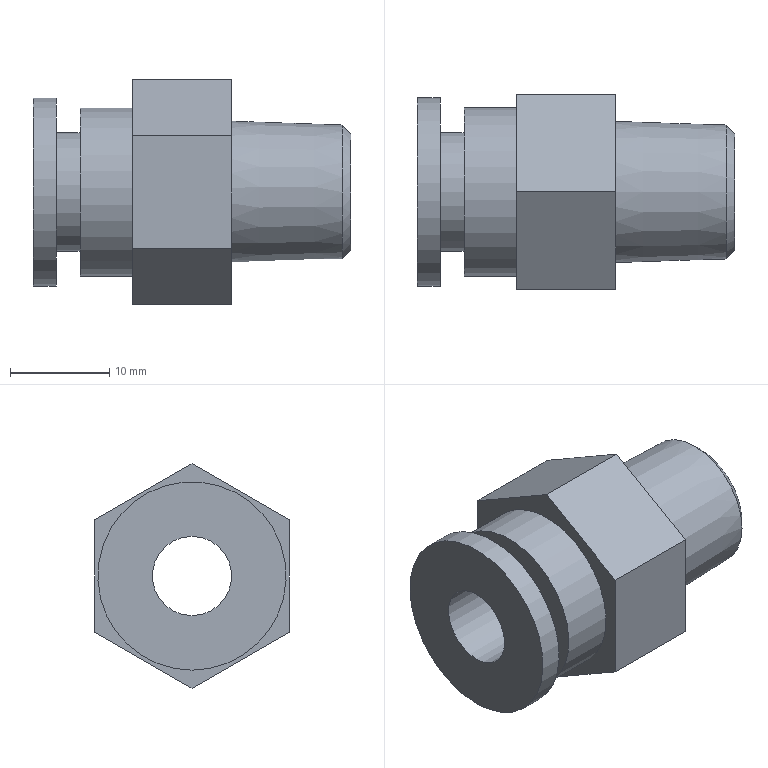Part | NX | features solid 2 | 1 solid | 18 faces | box 32 x 19.63 x 22.667 mm | volume 5655 mm3 | plane 12 | cylinder 4 | cone 2 | commonest cylinder face diameters 8 x1 12 x1 17 x1 19 x1
STEP:
#1=CARTESIAN_POINT('',(-113.,-72.,-29.095));
#2=VERTEX_POINT('',#1);
#3=CARTESIAN_POINT('',(-113.,-72.,-35.));
#4=DIRECTION('',(1.,0.,0.));
#5=DIRECTION('',(0.,0.,1.));
#6=AXIS2_PLACEMENT_3D('',#3,#4,#5);
#7=CIRCLE('',#6,5.905);
#8=EDGE_CURVE('',#2,#2,#7,.T.);
#9=ORIENTED_EDGE('',*,*,#8,.T.);
#10=EDGE_LOOP('',(#9));
#11=FACE_BOUND('',#10,.T.);
#12=CARTESIAN_POINT('',(-113.,-72.,-39.));
#13=VERTEX_POINT('',#12);
#14=CARTESIAN_POINT('',(-113.,-72.,-35.));
#15=DIRECTION('',(1.,0.,0.));
#16=DIRECTION('',(0.,0.,-1.));
#17=AXIS2_PLACEMENT_3D('',#14,#15,#16);
#18=CIRCLE('',#17,4.);
#19=EDGE_CURVE('',#13,#13,#18,.T.);
#20=ORIENTED_EDGE('',*,*,#19,.F.);
#21=EDGE_LOOP('',(#20));
#22=FACE_BOUND('',#21,.T.);
#23=CARTESIAN_POINT('',(-113.,-72.,-35.));
#24=DIRECTION('',(1.,0.,0.));
#25=DIRECTION('',(0.,0.,1.));
#26=AXIS2_PLACEMENT_3D('',#23,#24,#25);
#27=PLANE('',#26);
#28=ADVANCED_FACE('',(#11,#22),#27,.T.);
#29=CARTESIAN_POINT('',(-145.,-72.,-44.5));
#30=VERTEX_POINT('',#29);
#31=CARTESIAN_POINT('',(-145.,-72.,-35.));
#32=DIRECTION('',(-1.,0.,0.));
#33=DIRECTION('',(0.,0.,-1.));
#34=AXIS2_PLACEMENT_3D('',#31,#32,#33);
#35=CIRCLE('',#34,9.5);
#36=EDGE_CURVE('',#30,#30,#35,.T.);
#37=ORIENTED_EDGE('',*,*,#36,.T.);
#38=EDGE_LOOP('',(#37));
#39=FACE_BOUND('',#38,.T.);
#40=CARTESIAN_POINT('',(-145.,-72.,-39.));
#41=VERTEX_POINT('',#40);
#42=CARTESIAN_POINT('',(-145.,-72.,-35.));
#43=DIRECTION('',(-1.,0.,0.));
#44=DIRECTION('',(0.,0.,-1.));
#45=AXIS2_PLACEMENT_3D('',#42,#43,#44);
#46=CIRCLE('',#45,4.);
#47=EDGE_CURVE('',#41,#41,#46,.T.);
#48=ORIENTED_EDGE('',*,*,#47,.F.);
#49=EDGE_LOOP('',(#48));
#50=FACE_BOUND('',#49,.T.);
#51=CARTESIAN_POINT('',(-145.,-72.,-35.));
#52=DIRECTION('',(-1.,0.,0.));
#53=DIRECTION('',(0.,0.,-1.));
#54=AXIS2_PLACEMENT_3D('',#51,#52,#53);
#55=PLANE('',#54);
#56=ADVANCED_FACE('',(#39,#50),#55,.T.);
#57=ORIENTED_EDGE('',*,*,#8,.F.);
#58=EDGE_LOOP('',(#57));
#59=FACE_BOUND('',#58,.T.);
#60=CARTESIAN_POINT('',(-113.86,-72.,-28.24));
#61=VERTEX_POINT('',#60);
#62=CARTESIAN_POINT('',(-113.86,-72.,-35.));
#63=DIRECTION('',(1.,0.,0.));
#64=DIRECTION('',(0.,0.,1.));
#65=AXIS2_PLACEMENT_3D('',#62,#63,#64);
#66=CIRCLE('',#65,6.76);
#67=EDGE_CURVE('',#61,#61,#66,.T.);
#68=ORIENTED_EDGE('',*,*,#67,.T.);
#69=EDGE_LOOP('',(#68));
#70=FACE_BOUND('',#69,.T.);
#71=CARTESIAN_POINT('',(-113.,-72.,-35.));
#72=DIRECTION('',(-1.,0.,0.));
#73=DIRECTION('',(0.,0.,1.));
#74=AXIS2_PLACEMENT_3D('',#71,#72,#73);
#75=CONICAL_SURFACE('',#74,5.905,0.7825);
#76=ADVANCED_FACE('',(#59,#70),#75,.T.);
#77=ORIENTED_EDGE('',*,*,#67,.F.);
#78=EDGE_LOOP('',(#77));
#79=FACE_BOUND('',#78,.T.);
#80=CARTESIAN_POINT('',(-125.,-72.,-27.86));
#81=VERTEX_POINT('',#80);
#82=CARTESIAN_POINT('',(-125.,-72.,-35.));
#83=DIRECTION('',(-1.,0.,0.));
#84=DIRECTION('',(0.,0.,1.));
#85=AXIS2_PLACEMENT_3D('',#82,#83,#84);
#86=CIRCLE('',#85,7.14);
#87=EDGE_CURVE('',#81,#81,#86,.T.);
#88=ORIENTED_EDGE('',*,*,#87,.F.);
#89=EDGE_LOOP('',(#88));
#90=FACE_BOUND('',#89,.T.);
#91=CARTESIAN_POINT('',(-113.86,-72.,-35.));
#92=DIRECTION('',(-1.,0.,0.));
#93=DIRECTION('',(0.,0.,1.));
#94=AXIS2_PLACEMENT_3D('',#91,#92,#93);
#95=CONICAL_SURFACE('',#94,6.76,0.0341);
#96=ADVANCED_FACE('',(#79,#90),#95,.T.);
#97=CARTESIAN_POINT('',(-125.,-72.,-46.333));
#98=VERTEX_POINT('',#97);
#99=CARTESIAN_POINT('',(-125.,-62.185,-40.667));
#100=VERTEX_POINT('',#99);
#101=CARTESIAN_POINT('',(-125.,-72.,-46.333));
#102=DIRECTION('',(0.,0.866,0.5));
#103=VECTOR('',#102,1000.);
#104=LINE('',#101,#103);
#105=EDGE_CURVE('',#98,#100,#104,.T.);
#106=ORIENTED_EDGE('',*,*,#105,.T.);
#107=CARTESIAN_POINT('',(-125.,-62.185,-29.333));
#108=VERTEX_POINT('',#107);
#109=CARTESIAN_POINT('',(-125.,-62.185,-40.667));
#110=DIRECTION('',(0.,0.,1.));
#111=VECTOR('',#110,1000.);
#112=LINE('',#109,#111);
#113=EDGE_CURVE('',#100,#108,#112,.T.);
#114=ORIENTED_EDGE('',*,*,#113,.T.);
#115=CARTESIAN_POINT('',(-125.,-72.,-23.667));
#116=VERTEX_POINT('',#115);
#117=CARTESIAN_POINT('',(-125.,-62.185,-29.333));
#118=DIRECTION('',(0.,-0.866,0.5));
#119=VECTOR('',#118,1000.);
#120=LINE('',#117,#119);
#121=EDGE_CURVE('',#108,#116,#120,.T.);
#122=ORIENTED_EDGE('',*,*,#121,.T.);
#123=CARTESIAN_POINT('',(-125.,-81.815,-29.333));
#124=VERTEX_POINT('',#123);
#125=CARTESIAN_POINT('',(-125.,-72.,-23.667));
#126=DIRECTION('',(0.,-0.866,-0.5));
#127=VECTOR('',#126,1000.);
#128=LINE('',#125,#127);
#129=EDGE_CURVE('',#116,#124,#128,.T.);
#130=ORIENTED_EDGE('',*,*,#129,.T.);
#131=CARTESIAN_POINT('',(-125.,-81.815,-40.667));
#132=VERTEX_POINT('',#131);
#133=CARTESIAN_POINT('',(-125.,-81.815,-29.333));
#134=DIRECTION('',(0.,0.,-1.));
#135=VECTOR('',#134,1000.);
#136=LINE('',#133,#135);
#137=EDGE_CURVE('',#124,#132,#136,.T.);
#138=ORIENTED_EDGE('',*,*,#137,.T.);
#139=CARTESIAN_POINT('',(-125.,-81.815,-40.667));
#140=DIRECTION('',(0.,0.866,-0.5));
#141=VECTOR('',#140,1000.);
#142=LINE('',#139,#141);
#143=EDGE_CURVE('',#132,#98,#142,.T.);
#144=ORIENTED_EDGE('',*,*,#143,.T.);
#145=EDGE_LOOP('',(#106,#114,#122,#130,#138,#144));
#146=FACE_BOUND('',#145,.T.);
#147=ORIENTED_EDGE('',*,*,#87,.T.);
#148=EDGE_LOOP('',(#147));
#149=FACE_BOUND('',#148,.T.);
#150=CARTESIAN_POINT('',(-125.,-72.,-35.));
#151=DIRECTION('',(1.,0.,0.));
#152=DIRECTION('',(0.,0.,1.));
#153=AXIS2_PLACEMENT_3D('',#150,#151,#152);
#154=PLANE('',#153);
#155=ADVANCED_FACE('',(#146,#149),#154,.T.);
#156=CARTESIAN_POINT('',(-135.,-81.815,-40.667));
#157=VERTEX_POINT('',#156);
#158=CARTESIAN_POINT('',(-135.,-72.,-46.333));
#159=VERTEX_POINT('',#158);
#160=CARTESIAN_POINT('',(-135.,-81.815,-40.667));
#161=DIRECTION('',(0.,0.866,-0.5));
#162=VECTOR('',#161,1000.);
#163=LINE('',#160,#162);
#164=EDGE_CURVE('',#157,#159,#163,.T.);
#165=ORIENTED_EDGE('',*,*,#164,.T.);
#166=CARTESIAN_POINT('',(-125.,-72.,-46.333));
#167=DIRECTION('',(-1.,0.,0.));
#168=VECTOR('',#167,1000.);
#169=LINE('',#166,#168);
#170=EDGE_CURVE('',#98,#159,#169,.T.);
#171=ORIENTED_EDGE('',*,*,#170,.F.);
#172=ORIENTED_EDGE('',*,*,#143,.F.);
#173=CARTESIAN_POINT('',(-125.,-81.815,-40.667));
#174=DIRECTION('',(-1.,0.,0.));
#175=VECTOR('',#174,1000.);
#176=LINE('',#173,#175);
#177=EDGE_CURVE('',#132,#157,#176,.T.);
#178=ORIENTED_EDGE('',*,*,#177,.T.);
#179=EDGE_LOOP('',(#165,#171,#172,#178));
#180=FACE_BOUND('',#179,.T.);
#181=CARTESIAN_POINT('',(-130.,-76.907,-43.5));
#182=DIRECTION('',(0.,-0.5,-0.866));
#183=DIRECTION('',(0.,0.866,-0.5));
#184=AXIS2_PLACEMENT_3D('',#181,#182,#183);
#185=PLANE('',#184);
#186=ADVANCED_FACE('',(#180),#185,.T.);
#187=CARTESIAN_POINT('',(-135.,-81.815,-29.333));
#188=VERTEX_POINT('',#187);
#189=CARTESIAN_POINT('',(-135.,-81.815,-29.333));
#190=DIRECTION('',(0.,0.,-1.));
#191=VECTOR('',#190,1000.);
#192=LINE('',#189,#191);
#193=EDGE_CURVE('',#188,#157,#192,.T.);
#194=ORIENTED_EDGE('',*,*,#193,.T.);
#195=ORIENTED_EDGE('',*,*,#177,.F.);
#196=ORIENTED_EDGE('',*,*,#137,.F.);
#197=CARTESIAN_POINT('',(-125.,-81.815,-29.333));
#198=DIRECTION('',(-1.,0.,0.));
#199=VECTOR('',#198,1000.);
#200=LINE('',#197,#199);
#201=EDGE_CURVE('',#124,#188,#200,.T.);
#202=ORIENTED_EDGE('',*,*,#201,.T.);
#203=EDGE_LOOP('',(#194,#195,#196,#202));
#204=FACE_BOUND('',#203,.T.);
#205=CARTESIAN_POINT('',(-130.,-81.815,-35.));
#206=DIRECTION('',(0.,-1.,0.));
#207=DIRECTION('',(0.,0.,-1.));
#208=AXIS2_PLACEMENT_3D('',#205,#206,#207);
#209=PLANE('',#208);
#210=ADVANCED_FACE('',(#204),#209,.T.);
#211=CARTESIAN_POINT('',(-135.,-72.,-23.667));
#212=VERTEX_POINT('',#211);
#213=CARTESIAN_POINT('',(-135.,-72.,-23.667));
#214=DIRECTION('',(0.,-0.866,-0.5));
#215=VECTOR('',#214,1000.);
#216=LINE('',#213,#215);
#217=EDGE_CURVE('',#212,#188,#216,.T.);
#218=ORIENTED_EDGE('',*,*,#217,.T.);
#219=ORIENTED_EDGE('',*,*,#201,.F.);
#220=ORIENTED_EDGE('',*,*,#129,.F.);
#221=CARTESIAN_POINT('',(-125.,-72.,-23.667));
#222=DIRECTION('',(-1.,0.,0.));
#223=VECTOR('',#222,1000.);
#224=LINE('',#221,#223);
#225=EDGE_CURVE('',#116,#212,#224,.T.);
#226=ORIENTED_EDGE('',*,*,#225,.T.);
#227=EDGE_LOOP('',(#218,#219,#220,#226));
#228=FACE_BOUND('',#227,.T.);
#229=CARTESIAN_POINT('',(-130.,-76.907,-26.5));
#230=DIRECTION('',(0.,-0.5,0.866));
#231=DIRECTION('',(0.,-0.866,-0.5));
#232=AXIS2_PLACEMENT_3D('',#229,#230,#231);
#233=PLANE('',#232);
#234=ADVANCED_FACE('',(#228),#233,.T.);
#235=CARTESIAN_POINT('',(-135.,-62.185,-29.333));
#236=VERTEX_POINT('',#235);
#237=CARTESIAN_POINT('',(-135.,-62.185,-29.333));
#238=DIRECTION('',(0.,-0.866,0.5));
#239=VECTOR('',#238,1000.);
#240=LINE('',#237,#239);
#241=EDGE_CURVE('',#236,#212,#240,.T.);
#242=ORIENTED_EDGE('',*,*,#241,.T.);
#243=ORIENTED_EDGE('',*,*,#225,.F.);
#244=ORIENTED_EDGE('',*,*,#121,.F.);
#245=CARTESIAN_POINT('',(-125.,-62.185,-29.333));
#246=DIRECTION('',(-1.,0.,0.));
#247=VECTOR('',#246,1000.);
#248=LINE('',#245,#247);
#249=EDGE_CURVE('',#108,#236,#248,.T.);
#250=ORIENTED_EDGE('',*,*,#249,.T.);
#251=EDGE_LOOP('',(#242,#243,#244,#250));
#252=FACE_BOUND('',#251,.T.);
#253=CARTESIAN_POINT('',(-130.,-67.093,-26.5));
#254=DIRECTION('',(0.,0.5,0.866));
#255=DIRECTION('',(0.,-0.866,0.5));
#256=AXIS2_PLACEMENT_3D('',#253,#254,#255);
#257=PLANE('',#256);
#258=ADVANCED_FACE('',(#252),#257,.T.);
#259=CARTESIAN_POINT('',(-135.,-62.185,-40.667));
#260=VERTEX_POINT('',#259);
#261=CARTESIAN_POINT('',(-135.,-62.185,-40.667));
#262=DIRECTION('',(0.,0.,1.));
#263=VECTOR('',#262,1000.);
#264=LINE('',#261,#263);
#265=EDGE_CURVE('',#260,#236,#264,.T.);
#266=ORIENTED_EDGE('',*,*,#265,.T.);
#267=ORIENTED_EDGE('',*,*,#249,.F.);
#268=ORIENTED_EDGE('',*,*,#113,.F.);
#269=CARTESIAN_POINT('',(-125.,-62.185,-40.667));
#270=DIRECTION('',(-1.,0.,0.));
#271=VECTOR('',#270,1000.);
#272=LINE('',#269,#271);
#273=EDGE_CURVE('',#100,#260,#272,.T.);
#274=ORIENTED_EDGE('',*,*,#273,.T.);
#275=EDGE_LOOP('',(#266,#267,#268,#274));
#276=FACE_BOUND('',#275,.T.);
#277=CARTESIAN_POINT('',(-130.,-62.185,-35.));
#278=DIRECTION('',(0.,1.,0.));
#279=DIRECTION('',(1.,0.,0.));
#280=AXIS2_PLACEMENT_3D('',#277,#278,#279);
#281=PLANE('',#280);
#282=ADVANCED_FACE('',(#276),#281,.T.);
#283=CARTESIAN_POINT('',(-135.,-72.,-46.333));
#284=DIRECTION('',(0.,0.866,0.5));
#285=VECTOR('',#284,1000.);
#286=LINE('',#283,#285);
#287=EDGE_CURVE('',#159,#260,#286,.T.);
#288=ORIENTED_EDGE('',*,*,#287,.T.);
#289=ORIENTED_EDGE('',*,*,#273,.F.);
#290=ORIENTED_EDGE('',*,*,#105,.F.);
#291=ORIENTED_EDGE('',*,*,#170,.T.);
#292=EDGE_LOOP('',(#288,#289,#290,#291));
#293=FACE_BOUND('',#292,.T.);
#294=CARTESIAN_POINT('',(-130.,-67.093,-43.5));
#295=DIRECTION('',(0.,0.5,-0.866));
#296=DIRECTION('',(0.,0.866,0.5));
#297=AXIS2_PLACEMENT_3D('',#294,#295,#296);
#298=PLANE('',#297);
#299=ADVANCED_FACE('',(#293),#298,.T.);
#300=CARTESIAN_POINT('',(-135.,-72.,-43.5));
#301=VERTEX_POINT('',#300);
#302=CARTESIAN_POINT('',(-135.,-72.,-35.));
#303=DIRECTION('',(1.,0.,0.));
#304=DIRECTION('',(0.,0.,-1.));
#305=AXIS2_PLACEMENT_3D('',#302,#303,#304);
#306=CIRCLE('',#305,8.5);
#307=EDGE_CURVE('',#301,#301,#306,.T.);
#308=ORIENTED_EDGE('',*,*,#307,.T.);
#309=EDGE_LOOP('',(#308));
#310=FACE_BOUND('',#309,.T.);
#311=ORIENTED_EDGE('',*,*,#193,.F.);
#312=ORIENTED_EDGE('',*,*,#217,.F.);
#313=ORIENTED_EDGE('',*,*,#241,.F.);
#314=ORIENTED_EDGE('',*,*,#265,.F.);
#315=ORIENTED_EDGE('',*,*,#287,.F.);
#316=ORIENTED_EDGE('',*,*,#164,.F.);
#317=EDGE_LOOP('',(#311,#312,#313,#314,#315,#316));
#318=FACE_BOUND('',#317,.T.);
#319=CARTESIAN_POINT('',(-135.,-72.,-35.));
#320=DIRECTION('',(-1.,0.,0.));
#321=DIRECTION('',(0.,0.,-1.));
#322=AXIS2_PLACEMENT_3D('',#319,#320,#321);
#323=PLANE('',#322);
#324=ADVANCED_FACE('',(#310,#318),#323,.T.);
#325=CARTESIAN_POINT('',(-140.3,-72.,-41.));
#326=VERTEX_POINT('',#325);
#327=CARTESIAN_POINT('',(-140.3,-72.,-35.));
#328=DIRECTION('',(1.,0.,0.));
#329=DIRECTION('',(0.,0.,-1.));
#330=AXIS2_PLACEMENT_3D('',#327,#328,#329);
#331=CIRCLE('',#330,6.);
#332=EDGE_CURVE('',#326,#326,#331,.T.);
#333=ORIENTED_EDGE('',*,*,#332,.T.);
#334=EDGE_LOOP('',(#333));
#335=FACE_BOUND('',#334,.T.);
#336=CARTESIAN_POINT('',(-140.3,-72.,-43.5));
#337=VERTEX_POINT('',#336);
#338=CARTESIAN_POINT('',(-140.3,-72.,-35.));
#339=DIRECTION('',(-1.,0.,0.));
#340=DIRECTION('',(0.,0.,-1.));
#341=AXIS2_PLACEMENT_3D('',#338,#339,#340);
#342=CIRCLE('',#341,8.5);
#343=EDGE_CURVE('',#337,#337,#342,.T.);
#344=ORIENTED_EDGE('',*,*,#343,.T.);
#345=EDGE_LOOP('',(#344));
#346=FACE_BOUND('',#345,.T.);
#347=CARTESIAN_POINT('',(-140.3,-72.,-35.));
#348=DIRECTION('',(-1.,0.,0.));
#349=DIRECTION('',(0.,0.,-1.));
#350=AXIS2_PLACEMENT_3D('',#347,#348,#349);
#351=PLANE('',#350);
#352=ADVANCED_FACE('',(#335,#346),#351,.T.);
#353=ORIENTED_EDGE('',*,*,#343,.F.);
#354=EDGE_LOOP('',(#353));
#355=FACE_BOUND('',#354,.T.);
#356=ORIENTED_EDGE('',*,*,#307,.F.);
#357=EDGE_LOOP('',(#356));
#358=FACE_BOUND('',#357,.T.);
#359=CARTESIAN_POINT('',(-135.,-72.,-35.));
#360=DIRECTION('',(-1.,0.,0.));
#361=DIRECTION('',(0.,0.,-1.));
#362=AXIS2_PLACEMENT_3D('',#359,#360,#361);
#363=CYLINDRICAL_SURFACE('',#362,8.5);
#364=ADVANCED_FACE('',(#355,#358),#363,.T.);
#365=CARTESIAN_POINT('',(-142.7,-72.,-41.));
#366=VERTEX_POINT('',#365);
#367=CARTESIAN_POINT('',(-142.7,-72.,-35.));
#368=DIRECTION('',(-1.,0.,0.));
#369=DIRECTION('',(0.,0.,-1.));
#370=AXIS2_PLACEMENT_3D('',#367,#368,#369);
#371=CIRCLE('',#370,6.);
#372=EDGE_CURVE('',#366,#366,#371,.T.);
#373=ORIENTED_EDGE('',*,*,#372,.F.);
#374=EDGE_LOOP('',(#373));
#375=FACE_BOUND('',#374,.T.);
#376=ORIENTED_EDGE('',*,*,#332,.F.);
#377=EDGE_LOOP('',(#376));
#378=FACE_BOUND('',#377,.T.);
#379=CARTESIAN_POINT('',(-140.3,-72.,-35.));
#380=DIRECTION('',(-1.,0.,0.));
#381=DIRECTION('',(0.,0.,-1.));
#382=AXIS2_PLACEMENT_3D('',#379,#380,#381);
#383=CYLINDRICAL_SURFACE('',#382,6.);
#384=ADVANCED_FACE('',(#375,#378),#383,.T.);
#385=CARTESIAN_POINT('',(-142.7,-72.,-44.5));
#386=VERTEX_POINT('',#385);
#387=CARTESIAN_POINT('',(-142.7,-72.,-35.));
#388=DIRECTION('',(1.,0.,0.));
#389=DIRECTION('',(0.,0.,-1.));
#390=AXIS2_PLACEMENT_3D('',#387,#388,#389);
#391=CIRCLE('',#390,9.5);
#392=EDGE_CURVE('',#386,#386,#391,.T.);
#393=ORIENTED_EDGE('',*,*,#392,.T.);
#394=EDGE_LOOP('',(#393));
#395=FACE_BOUND('',#394,.T.);
#396=ORIENTED_EDGE('',*,*,#372,.T.);
#397=EDGE_LOOP('',(#396));
#398=FACE_BOUND('',#397,.T.);
#399=CARTESIAN_POINT('',(-142.7,-72.,-35.));
#400=DIRECTION('',(1.,0.,0.));
#401=DIRECTION('',(0.,0.,1.));
#402=AXIS2_PLACEMENT_3D('',#399,#400,#401);
#403=PLANE('',#402);
#404=ADVANCED_FACE('',(#395,#398),#403,.T.);
#405=ORIENTED_EDGE('',*,*,#36,.F.);
#406=EDGE_LOOP('',(#405));
#407=FACE_BOUND('',#406,.T.);
#408=ORIENTED_EDGE('',*,*,#392,.F.);
#409=EDGE_LOOP('',(#408));
#410=FACE_BOUND('',#409,.T.);
#411=CARTESIAN_POINT('',(-142.7,-72.,-35.));
#412=DIRECTION('',(-1.,0.,0.));
#413=DIRECTION('',(0.,0.,-1.));
#414=AXIS2_PLACEMENT_3D('',#411,#412,#413);
#415=CYLINDRICAL_SURFACE('',#414,9.5);
#416=ADVANCED_FACE('',(#407,#410),#415,.T.);
#417=ORIENTED_EDGE('',*,*,#47,.T.);
#418=EDGE_LOOP('',(#417));
#419=FACE_BOUND('',#418,.T.);
#420=ORIENTED_EDGE('',*,*,#19,.T.);
#421=EDGE_LOOP('',(#420));
#422=FACE_BOUND('',#421,.T.);
#423=CARTESIAN_POINT('',(-113.,-72.,-35.));
#424=DIRECTION('',(-1.,0.,0.));
#425=DIRECTION('',(0.,0.,-1.));
#426=AXIS2_PLACEMENT_3D('',#423,#424,#425);
#427=CYLINDRICAL_SURFACE('',#426,4.);
#428=ADVANCED_FACE('',(#419,#422),#427,.F.);
#429=CLOSED_SHELL('',(#28,#56,#76,#96,#155,#186,#210,#234,#258,#282,#299,#324,#352,#364,#384,#404,#416,#428));
#430=MANIFOLD_SOLID_BREP('',#429);
#431=(LENGTH_UNIT()NAMED_UNIT(*)SI_UNIT(.MILLI.,.METRE.));
#432=UNCERTAINTY_MEASURE_WITH_UNIT(LENGTH_MEASURE(0.00001),#431,'','');
#433=(NAMED_UNIT(*)PLANE_ANGLE_UNIT()SI_UNIT($,.RADIAN.));
#434=(NAMED_UNIT(*)SI_UNIT($,.STERADIAN.)SOLID_ANGLE_UNIT());
#435=(GEOMETRIC_REPRESENTATION_CONTEXT(3)GLOBAL_UNCERTAINTY_ASSIGNED_CONTEXT((#432))GLOBAL_UNIT_ASSIGNED_CONTEXT((#431,#433,#434))REPRESENTATION_CONTEXT('',''));
#436=ADVANCED_BREP_SHAPE_REPRESENTATION('',(#430),#435);